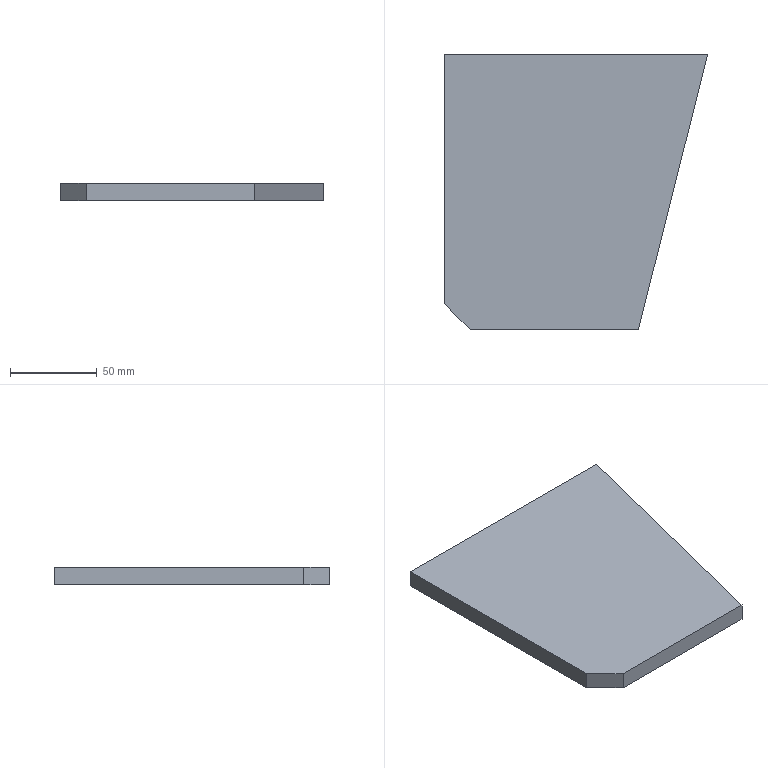Part | STEP file | 03-Rib plate | 1 solid | 7 faces | box 152 x 159 x 10 mm | volume 208755 mm3 | plane 7
STEP:
#1=CARTESIAN_POINT('',(0.,0.,0.));
#2=DIRECTION('',(0.,0.,1.));
#3=DIRECTION('',(1.,0.,0.));
#4=AXIS2_PLACEMENT_3D('',#1,#2,#3);
#5=CARTESIAN_POINT('',(0.,0.,0.));
#6=VERTEX_POINT('',#5);
#7=CARTESIAN_POINT('',(0.,-144.,0.));
#8=VERTEX_POINT('',#7);
#9=CARTESIAN_POINT('',(0.,0.,0.));
#10=DIRECTION('',(0.,-1.,0.));
#11=VECTOR('',#10,1.);
#12=LINE('',#9,#11);
#13=CARTESIAN_POINT('',(0.,0.,10.));
#14=DIRECTION('',(1.,0.,0.));
#15=DIRECTION('',(0.,1.,0.));
#16=AXIS2_PLACEMENT_3D('',#13,#14,#15);
#17=PLANE('',#16);
#18=CARTESIAN_POINT('',(0.,-10.));
#19=DIRECTION('',(-1.,0.));
#20=VECTOR('',#19,1.);
#21=LINE('',#18,#20);
#22=(GEOMETRIC_REPRESENTATION_CONTEXT(2)PARAMETRIC_REPRESENTATION_CONTEXT()REPRESENTATION_CONTEXT('',''));
#23=DEFINITIONAL_REPRESENTATION('',(#21),#22);
#24=PCURVE('',#17,#23);
#25=CARTESIAN_POINT('',(0.,0.,0.));
#26=DIRECTION('',(0.,0.,1.));
#27=DIRECTION('',(1.,0.,0.));
#28=AXIS2_PLACEMENT_3D('',#25,#26,#27);
#29=PLANE('',#28);
#30=CARTESIAN_POINT('',(0.,0.));
#31=DIRECTION('',(0.,-1.));
#32=VECTOR('',#31,1.);
#33=LINE('',#30,#32);
#34=(GEOMETRIC_REPRESENTATION_CONTEXT(2)PARAMETRIC_REPRESENTATION_CONTEXT()REPRESENTATION_CONTEXT('',''));
#35=DEFINITIONAL_REPRESENTATION('',(#33),#34);
#36=PCURVE('',#29,#35);
#37=SURFACE_CURVE('',#12,(#24,#36),.PCURVE_S1.);
#38=EDGE_CURVE('',#6,#8,#37,.T.);
#39=ORIENTED_EDGE('',*,*,#38,.T.);
#40=CARTESIAN_POINT('',(0.,-144.,10.));
#41=VERTEX_POINT('',#40);
#42=CARTESIAN_POINT('',(0.,-144.,10.));
#43=DIRECTION('',(0.,0.,-1.));
#44=VECTOR('',#43,1.);
#45=LINE('',#42,#44);
#46=CARTESIAN_POINT('',(-144.,0.));
#47=DIRECTION('',(0.,-1.));
#48=VECTOR('',#47,1.);
#49=LINE('',#46,#48);
#50=(GEOMETRIC_REPRESENTATION_CONTEXT(2)PARAMETRIC_REPRESENTATION_CONTEXT()REPRESENTATION_CONTEXT('',''));
#51=DEFINITIONAL_REPRESENTATION('',(#49),#50);
#52=PCURVE('',#17,#51);
#53=CARTESIAN_POINT('',(0.,-144.,10.));
#54=DIRECTION('',(0.7071,0.7071,0.));
#55=DIRECTION('',(-0.7071,0.7071,0.));
#56=AXIS2_PLACEMENT_3D('',#53,#54,#55);
#57=PLANE('',#56);
#58=CARTESIAN_POINT('',(0.,0.));
#59=DIRECTION('',(0.,-1.));
#60=VECTOR('',#59,1.);
#61=LINE('',#58,#60);
#62=(GEOMETRIC_REPRESENTATION_CONTEXT(2)PARAMETRIC_REPRESENTATION_CONTEXT()REPRESENTATION_CONTEXT('',''));
#63=DEFINITIONAL_REPRESENTATION('',(#61),#62);
#64=PCURVE('',#57,#63);
#65=SURFACE_CURVE('',#45,(#52,#64),.PCURVE_S1.);
#66=EDGE_CURVE('',#41,#8,#65,.T.);
#67=ORIENTED_EDGE('',*,*,#66,.F.);
#68=CARTESIAN_POINT('',(0.,0.,10.));
#69=VERTEX_POINT('',#68);
#70=CARTESIAN_POINT('',(0.,0.,10.));
#71=DIRECTION('',(0.,-1.,0.));
#72=VECTOR('',#71,1.);
#73=LINE('',#70,#72);
#74=CARTESIAN_POINT('',(0.,0.));
#75=DIRECTION('',(-1.,0.));
#76=VECTOR('',#75,1.);
#77=LINE('',#74,#76);
#78=(GEOMETRIC_REPRESENTATION_CONTEXT(2)PARAMETRIC_REPRESENTATION_CONTEXT()REPRESENTATION_CONTEXT('',''));
#79=DEFINITIONAL_REPRESENTATION('',(#77),#78);
#80=PCURVE('',#17,#79);
#81=CARTESIAN_POINT('',(0.,0.,10.));
#82=DIRECTION('',(0.,0.,1.));
#83=DIRECTION('',(1.,0.,0.));
#84=AXIS2_PLACEMENT_3D('',#81,#82,#83);
#85=PLANE('',#84);
#86=CARTESIAN_POINT('',(0.,0.));
#87=DIRECTION('',(0.,-1.));
#88=VECTOR('',#87,1.);
#89=LINE('',#86,#88);
#90=(GEOMETRIC_REPRESENTATION_CONTEXT(2)PARAMETRIC_REPRESENTATION_CONTEXT()REPRESENTATION_CONTEXT('',''));
#91=DEFINITIONAL_REPRESENTATION('',(#89),#90);
#92=PCURVE('',#85,#91);
#93=SURFACE_CURVE('',#73,(#80,#92),.PCURVE_S1.);
#94=EDGE_CURVE('',#69,#41,#93,.T.);
#95=ORIENTED_EDGE('',*,*,#94,.F.);
#96=CARTESIAN_POINT('',(0.,0.,10.));
#97=DIRECTION('',(0.,0.,-1.));
#98=VECTOR('',#97,1.);
#99=LINE('',#96,#98);
#100=CARTESIAN_POINT('',(0.,0.));
#101=DIRECTION('',(0.,-1.));
#102=VECTOR('',#101,1.);
#103=LINE('',#100,#102);
#104=(GEOMETRIC_REPRESENTATION_CONTEXT(2)PARAMETRIC_REPRESENTATION_CONTEXT()REPRESENTATION_CONTEXT('',''));
#105=DEFINITIONAL_REPRESENTATION('',(#103),#104);
#106=PCURVE('',#17,#105);
#107=CARTESIAN_POINT('',(0.,0.,10.));
#108=DIRECTION('',(0.,-1.,0.));
#109=DIRECTION('',(0.,0.,-1.));
#110=AXIS2_PLACEMENT_3D('',#107,#108,#109);
#111=PLANE('',#110);
#112=CARTESIAN_POINT('',(0.,0.));
#113=DIRECTION('',(1.,0.));
#114=VECTOR('',#113,1.);
#115=LINE('',#112,#114);
#116=(GEOMETRIC_REPRESENTATION_CONTEXT(2)PARAMETRIC_REPRESENTATION_CONTEXT()REPRESENTATION_CONTEXT('',''));
#117=DEFINITIONAL_REPRESENTATION('',(#115),#116);
#118=PCURVE('',#111,#117);
#119=SURFACE_CURVE('',#99,(#106,#118),.PCURVE_S1.);
#120=EDGE_CURVE('',#69,#6,#119,.T.);
#121=ORIENTED_EDGE('',*,*,#120,.T.);
#122=EDGE_LOOP('',(#39,#67,#95,#121));
#123=FACE_BOUND('',#122,.T.);
#124=ADVANCED_FACE('',(#123),#17,.F.);
#125=CARTESIAN_POINT('',(15.,-159.,0.));
#126=VERTEX_POINT('',#125);
#127=CARTESIAN_POINT('',(0.,-144.,0.));
#128=DIRECTION('',(0.7071,-0.7071,0.));
#129=VECTOR('',#128,1.);
#130=LINE('',#127,#129);
#131=CARTESIAN_POINT('',(0.,-10.));
#132=DIRECTION('',(-1.,0.));
#133=VECTOR('',#132,1.);
#134=LINE('',#131,#133);
#135=(GEOMETRIC_REPRESENTATION_CONTEXT(2)PARAMETRIC_REPRESENTATION_CONTEXT()REPRESENTATION_CONTEXT('',''));
#136=DEFINITIONAL_REPRESENTATION('',(#134),#135);
#137=PCURVE('',#57,#136);
#138=CARTESIAN_POINT('',(0.,-144.));
#139=DIRECTION('',(0.7071,-0.7071));
#140=VECTOR('',#139,1.);
#141=LINE('',#138,#140);
#142=(GEOMETRIC_REPRESENTATION_CONTEXT(2)PARAMETRIC_REPRESENTATION_CONTEXT()REPRESENTATION_CONTEXT('',''));
#143=DEFINITIONAL_REPRESENTATION('',(#141),#142);
#144=PCURVE('',#29,#143);
#145=SURFACE_CURVE('',#130,(#137,#144),.PCURVE_S1.);
#146=EDGE_CURVE('',#8,#126,#145,.T.);
#147=ORIENTED_EDGE('',*,*,#146,.T.);
#148=CARTESIAN_POINT('',(15.,-159.,10.));
#149=VERTEX_POINT('',#148);
#150=CARTESIAN_POINT('',(15.,-159.,10.));
#151=DIRECTION('',(0.,0.,-1.));
#152=VECTOR('',#151,1.);
#153=LINE('',#150,#152);
#154=CARTESIAN_POINT('',(-21.213,0.));
#155=DIRECTION('',(0.,-1.));
#156=VECTOR('',#155,1.);
#157=LINE('',#154,#156);
#158=(GEOMETRIC_REPRESENTATION_CONTEXT(2)PARAMETRIC_REPRESENTATION_CONTEXT()REPRESENTATION_CONTEXT('',''));
#159=DEFINITIONAL_REPRESENTATION('',(#157),#158);
#160=PCURVE('',#57,#159);
#161=CARTESIAN_POINT('',(15.,-159.,10.));
#162=DIRECTION('',(0.,1.,0.));
#163=DIRECTION('',(0.,0.,1.));
#164=AXIS2_PLACEMENT_3D('',#161,#162,#163);
#165=PLANE('',#164);
#166=CARTESIAN_POINT('',(0.,0.));
#167=DIRECTION('',(-1.,0.));
#168=VECTOR('',#167,1.);
#169=LINE('',#166,#168);
#170=(GEOMETRIC_REPRESENTATION_CONTEXT(2)PARAMETRIC_REPRESENTATION_CONTEXT()REPRESENTATION_CONTEXT('',''));
#171=DEFINITIONAL_REPRESENTATION('',(#169),#170);
#172=PCURVE('',#165,#171);
#173=SURFACE_CURVE('',#153,(#160,#172),.PCURVE_S1.);
#174=EDGE_CURVE('',#149,#126,#173,.T.);
#175=ORIENTED_EDGE('',*,*,#174,.F.);
#176=CARTESIAN_POINT('',(0.,-144.,10.));
#177=DIRECTION('',(0.7071,-0.7071,0.));
#178=VECTOR('',#177,1.);
#179=LINE('',#176,#178);
#180=CARTESIAN_POINT('',(0.,0.));
#181=DIRECTION('',(-1.,0.));
#182=VECTOR('',#181,1.);
#183=LINE('',#180,#182);
#184=(GEOMETRIC_REPRESENTATION_CONTEXT(2)PARAMETRIC_REPRESENTATION_CONTEXT()REPRESENTATION_CONTEXT('',''));
#185=DEFINITIONAL_REPRESENTATION('',(#183),#184);
#186=PCURVE('',#57,#185);
#187=CARTESIAN_POINT('',(0.,-144.));
#188=DIRECTION('',(0.7071,-0.7071));
#189=VECTOR('',#188,1.);
#190=LINE('',#187,#189);
#191=(GEOMETRIC_REPRESENTATION_CONTEXT(2)PARAMETRIC_REPRESENTATION_CONTEXT()REPRESENTATION_CONTEXT('',''));
#192=DEFINITIONAL_REPRESENTATION('',(#190),#191);
#193=PCURVE('',#85,#192);
#194=SURFACE_CURVE('',#179,(#186,#193),.PCURVE_S1.);
#195=EDGE_CURVE('',#41,#149,#194,.T.);
#196=ORIENTED_EDGE('',*,*,#195,.F.);
#197=ORIENTED_EDGE('',*,*,#66,.T.);
#198=EDGE_LOOP('',(#147,#175,#196,#197));
#199=FACE_BOUND('',#198,.T.);
#200=ADVANCED_FACE('',(#199),#57,.F.);
#201=CARTESIAN_POINT('',(112.,-159.,0.));
#202=VERTEX_POINT('',#201);
#203=CARTESIAN_POINT('',(15.,-159.,0.));
#204=DIRECTION('',(1.,0.,0.));
#205=VECTOR('',#204,1.);
#206=LINE('',#203,#205);
#207=CARTESIAN_POINT('',(-10.,0.));
#208=DIRECTION('',(0.,1.));
#209=VECTOR('',#208,1.);
#210=LINE('',#207,#209);
#211=(GEOMETRIC_REPRESENTATION_CONTEXT(2)PARAMETRIC_REPRESENTATION_CONTEXT()REPRESENTATION_CONTEXT('',''));
#212=DEFINITIONAL_REPRESENTATION('',(#210),#211);
#213=PCURVE('',#165,#212);
#214=CARTESIAN_POINT('',(15.,-159.));
#215=DIRECTION('',(1.,0.));
#216=VECTOR('',#215,1.);
#217=LINE('',#214,#216);
#218=(GEOMETRIC_REPRESENTATION_CONTEXT(2)PARAMETRIC_REPRESENTATION_CONTEXT()REPRESENTATION_CONTEXT('',''));
#219=DEFINITIONAL_REPRESENTATION('',(#217),#218);
#220=PCURVE('',#29,#219);
#221=SURFACE_CURVE('',#206,(#213,#220),.PCURVE_S1.);
#222=EDGE_CURVE('',#126,#202,#221,.T.);
#223=ORIENTED_EDGE('',*,*,#222,.T.);
#224=CARTESIAN_POINT('',(112.,-159.,10.));
#225=VERTEX_POINT('',#224);
#226=CARTESIAN_POINT('',(112.,-159.,10.));
#227=DIRECTION('',(0.,0.,-1.));
#228=VECTOR('',#227,1.);
#229=LINE('',#226,#228);
#230=CARTESIAN_POINT('',(0.,97.));
#231=DIRECTION('',(-1.,0.));
#232=VECTOR('',#231,1.);
#233=LINE('',#230,#232);
#234=(GEOMETRIC_REPRESENTATION_CONTEXT(2)PARAMETRIC_REPRESENTATION_CONTEXT()REPRESENTATION_CONTEXT('',''));
#235=DEFINITIONAL_REPRESENTATION('',(#233),#234);
#236=PCURVE('',#165,#235);
#237=CARTESIAN_POINT('',(152.,0.,10.));
#238=DIRECTION('',(-0.9698,0.244,0.));
#239=DIRECTION('',(-0.244,-0.9698,0.));
#240=AXIS2_PLACEMENT_3D('',#237,#238,#239);
#241=PLANE('',#240);
#242=CARTESIAN_POINT('',(163.954,0.));
#243=DIRECTION('',(0.,-1.));
#244=VECTOR('',#243,1.);
#245=LINE('',#242,#244);
#246=(GEOMETRIC_REPRESENTATION_CONTEXT(2)PARAMETRIC_REPRESENTATION_CONTEXT()REPRESENTATION_CONTEXT('',''));
#247=DEFINITIONAL_REPRESENTATION('',(#245),#246);
#248=PCURVE('',#241,#247);
#249=SURFACE_CURVE('',#229,(#236,#248),.PCURVE_S1.);
#250=EDGE_CURVE('',#225,#202,#249,.T.);
#251=ORIENTED_EDGE('',*,*,#250,.F.);
#252=CARTESIAN_POINT('',(15.,-159.,10.));
#253=DIRECTION('',(1.,0.,0.));
#254=VECTOR('',#253,1.);
#255=LINE('',#252,#254);
#256=CARTESIAN_POINT('',(0.,0.));
#257=DIRECTION('',(0.,1.));
#258=VECTOR('',#257,1.);
#259=LINE('',#256,#258);
#260=(GEOMETRIC_REPRESENTATION_CONTEXT(2)PARAMETRIC_REPRESENTATION_CONTEXT()REPRESENTATION_CONTEXT('',''));
#261=DEFINITIONAL_REPRESENTATION('',(#259),#260);
#262=PCURVE('',#165,#261);
#263=CARTESIAN_POINT('',(15.,-159.));
#264=DIRECTION('',(1.,0.));
#265=VECTOR('',#264,1.);
#266=LINE('',#263,#265);
#267=(GEOMETRIC_REPRESENTATION_CONTEXT(2)PARAMETRIC_REPRESENTATION_CONTEXT()REPRESENTATION_CONTEXT('',''));
#268=DEFINITIONAL_REPRESENTATION('',(#266),#267);
#269=PCURVE('',#85,#268);
#270=SURFACE_CURVE('',#255,(#262,#269),.PCURVE_S1.);
#271=EDGE_CURVE('',#149,#225,#270,.T.);
#272=ORIENTED_EDGE('',*,*,#271,.F.);
#273=ORIENTED_EDGE('',*,*,#174,.T.);
#274=EDGE_LOOP('',(#223,#251,#272,#273));
#275=FACE_BOUND('',#274,.T.);
#276=ADVANCED_FACE('',(#275),#165,.F.);
#277=CARTESIAN_POINT('',(152.,0.,0.));
#278=VERTEX_POINT('',#277);
#279=CARTESIAN_POINT('',(152.,0.,0.));
#280=DIRECTION('',(0.244,0.9698,0.));
#281=VECTOR('',#280,1.);
#282=LINE('',#279,#281);
#283=CARTESIAN_POINT('',(0.,-10.));
#284=DIRECTION('',(-1.,0.));
#285=VECTOR('',#284,1.);
#286=LINE('',#283,#285);
#287=(GEOMETRIC_REPRESENTATION_CONTEXT(2)PARAMETRIC_REPRESENTATION_CONTEXT()REPRESENTATION_CONTEXT('',''));
#288=DEFINITIONAL_REPRESENTATION('',(#286),#287);
#289=PCURVE('',#241,#288);
#290=CARTESIAN_POINT('',(152.,0.));
#291=DIRECTION('',(0.244,0.9698));
#292=VECTOR('',#291,1.);
#293=LINE('',#290,#292);
#294=(GEOMETRIC_REPRESENTATION_CONTEXT(2)PARAMETRIC_REPRESENTATION_CONTEXT()REPRESENTATION_CONTEXT('',''));
#295=DEFINITIONAL_REPRESENTATION('',(#293),#294);
#296=PCURVE('',#29,#295);
#297=SURFACE_CURVE('',#282,(#289,#296),.PCURVE_S1.);
#298=EDGE_CURVE('',#202,#278,#297,.T.);
#299=ORIENTED_EDGE('',*,*,#298,.T.);
#300=CARTESIAN_POINT('',(152.,0.,10.));
#301=VERTEX_POINT('',#300);
#302=CARTESIAN_POINT('',(152.,0.,10.));
#303=DIRECTION('',(0.,0.,-1.));
#304=VECTOR('',#303,1.);
#305=LINE('',#302,#304);
#306=CARTESIAN_POINT('',(0.,0.));
#307=DIRECTION('',(0.,-1.));
#308=VECTOR('',#307,1.);
#309=LINE('',#306,#308);
#310=(GEOMETRIC_REPRESENTATION_CONTEXT(2)PARAMETRIC_REPRESENTATION_CONTEXT()REPRESENTATION_CONTEXT('',''));
#311=DEFINITIONAL_REPRESENTATION('',(#309),#310);
#312=PCURVE('',#241,#311);
#313=CARTESIAN_POINT('',(0.,152.));
#314=DIRECTION('',(1.,0.));
#315=VECTOR('',#314,1.);
#316=LINE('',#313,#315);
#317=(GEOMETRIC_REPRESENTATION_CONTEXT(2)PARAMETRIC_REPRESENTATION_CONTEXT()REPRESENTATION_CONTEXT('',''));
#318=DEFINITIONAL_REPRESENTATION('',(#316),#317);
#319=PCURVE('',#111,#318);
#320=SURFACE_CURVE('',#305,(#312,#319),.PCURVE_S1.);
#321=EDGE_CURVE('',#301,#278,#320,.T.);
#322=ORIENTED_EDGE('',*,*,#321,.F.);
#323=CARTESIAN_POINT('',(152.,0.,10.));
#324=DIRECTION('',(0.244,0.9698,0.));
#325=VECTOR('',#324,1.);
#326=LINE('',#323,#325);
#327=CARTESIAN_POINT('',(0.,0.));
#328=DIRECTION('',(-1.,0.));
#329=VECTOR('',#328,1.);
#330=LINE('',#327,#329);
#331=(GEOMETRIC_REPRESENTATION_CONTEXT(2)PARAMETRIC_REPRESENTATION_CONTEXT()REPRESENTATION_CONTEXT('',''));
#332=DEFINITIONAL_REPRESENTATION('',(#330),#331);
#333=PCURVE('',#241,#332);
#334=CARTESIAN_POINT('',(152.,0.));
#335=DIRECTION('',(0.244,0.9698));
#336=VECTOR('',#335,1.);
#337=LINE('',#334,#336);
#338=(GEOMETRIC_REPRESENTATION_CONTEXT(2)PARAMETRIC_REPRESENTATION_CONTEXT()REPRESENTATION_CONTEXT('',''));
#339=DEFINITIONAL_REPRESENTATION('',(#337),#338);
#340=PCURVE('',#85,#339);
#341=SURFACE_CURVE('',#326,(#333,#340),.PCURVE_S1.);
#342=EDGE_CURVE('',#225,#301,#341,.T.);
#343=ORIENTED_EDGE('',*,*,#342,.F.);
#344=ORIENTED_EDGE('',*,*,#250,.T.);
#345=EDGE_LOOP('',(#299,#322,#343,#344));
#346=FACE_BOUND('',#345,.T.);
#347=ADVANCED_FACE('',(#346),#241,.F.);
#348=CARTESIAN_POINT('',(0.,0.,0.));
#349=DIRECTION('',(-1.,0.,0.));
#350=VECTOR('',#349,1.);
#351=LINE('',#348,#350);
#352=CARTESIAN_POINT('',(10.,0.));
#353=DIRECTION('',(0.,-1.));
#354=VECTOR('',#353,1.);
#355=LINE('',#352,#354);
#356=(GEOMETRIC_REPRESENTATION_CONTEXT(2)PARAMETRIC_REPRESENTATION_CONTEXT()REPRESENTATION_CONTEXT('',''));
#357=DEFINITIONAL_REPRESENTATION('',(#355),#356);
#358=PCURVE('',#111,#357);
#359=CARTESIAN_POINT('',(0.,0.));
#360=DIRECTION('',(-1.,0.));
#361=VECTOR('',#360,1.);
#362=LINE('',#359,#361);
#363=(GEOMETRIC_REPRESENTATION_CONTEXT(2)PARAMETRIC_REPRESENTATION_CONTEXT()REPRESENTATION_CONTEXT('',''));
#364=DEFINITIONAL_REPRESENTATION('',(#362),#363);
#365=PCURVE('',#29,#364);
#366=SURFACE_CURVE('',#351,(#358,#365),.PCURVE_S1.);
#367=EDGE_CURVE('',#278,#6,#366,.T.);
#368=ORIENTED_EDGE('',*,*,#367,.T.);
#369=ORIENTED_EDGE('',*,*,#120,.F.);
#370=CARTESIAN_POINT('',(0.,0.,10.));
#371=DIRECTION('',(-1.,0.,0.));
#372=VECTOR('',#371,1.);
#373=LINE('',#370,#372);
#374=CARTESIAN_POINT('',(0.,0.));
#375=DIRECTION('',(0.,-1.));
#376=VECTOR('',#375,1.);
#377=LINE('',#374,#376);
#378=(GEOMETRIC_REPRESENTATION_CONTEXT(2)PARAMETRIC_REPRESENTATION_CONTEXT()REPRESENTATION_CONTEXT('',''));
#379=DEFINITIONAL_REPRESENTATION('',(#377),#378);
#380=PCURVE('',#111,#379);
#381=CARTESIAN_POINT('',(0.,0.));
#382=DIRECTION('',(-1.,0.));
#383=VECTOR('',#382,1.);
#384=LINE('',#381,#383);
#385=(GEOMETRIC_REPRESENTATION_CONTEXT(2)PARAMETRIC_REPRESENTATION_CONTEXT()REPRESENTATION_CONTEXT('',''));
#386=DEFINITIONAL_REPRESENTATION('',(#384),#385);
#387=PCURVE('',#85,#386);
#388=SURFACE_CURVE('',#373,(#380,#387),.PCURVE_S1.);
#389=EDGE_CURVE('',#301,#69,#388,.T.);
#390=ORIENTED_EDGE('',*,*,#389,.F.);
#391=ORIENTED_EDGE('',*,*,#321,.T.);
#392=EDGE_LOOP('',(#368,#369,#390,#391));
#393=FACE_BOUND('',#392,.T.);
#394=ADVANCED_FACE('',(#393),#111,.F.);
#395=ORIENTED_EDGE('',*,*,#94,.T.);
#396=ORIENTED_EDGE('',*,*,#195,.T.);
#397=ORIENTED_EDGE('',*,*,#271,.T.);
#398=ORIENTED_EDGE('',*,*,#342,.T.);
#399=ORIENTED_EDGE('',*,*,#389,.T.);
#400=EDGE_LOOP('',(#395,#396,#397,#398,#399));
#401=FACE_BOUND('',#400,.T.);
#402=ADVANCED_FACE('',(#401),#85,.T.);
#403=ORIENTED_EDGE('',*,*,#38,.F.);
#404=ORIENTED_EDGE('',*,*,#367,.F.);
#405=ORIENTED_EDGE('',*,*,#298,.F.);
#406=ORIENTED_EDGE('',*,*,#222,.F.);
#407=ORIENTED_EDGE('',*,*,#146,.F.);
#408=EDGE_LOOP('',(#403,#404,#405,#406,#407));
#409=FACE_BOUND('',#408,.T.);
#410=ADVANCED_FACE('',(#409),#29,.F.);
#411=CLOSED_SHELL('',(#124,#200,#276,#347,#394,#402,#410));
#412=MANIFOLD_SOLID_BREP('',#411);
#413=(LENGTH_UNIT()NAMED_UNIT(*)SI_UNIT(.MILLI.,.METRE.));
#414=UNCERTAINTY_MEASURE_WITH_UNIT(LENGTH_MEASURE(0.0000001),#413,'','');
#415=(NAMED_UNIT(*)PLANE_ANGLE_UNIT()SI_UNIT($,.RADIAN.));
#416=(NAMED_UNIT(*)SI_UNIT($,.STERADIAN.)SOLID_ANGLE_UNIT());
#417=(GEOMETRIC_REPRESENTATION_CONTEXT(3)GLOBAL_UNCERTAINTY_ASSIGNED_CONTEXT((#414))GLOBAL_UNIT_ASSIGNED_CONTEXT((#413,#415,#416))REPRESENTATION_CONTEXT('',''));
#418=ADVANCED_BREP_SHAPE_REPRESENTATION('',(#4,#412),#417);